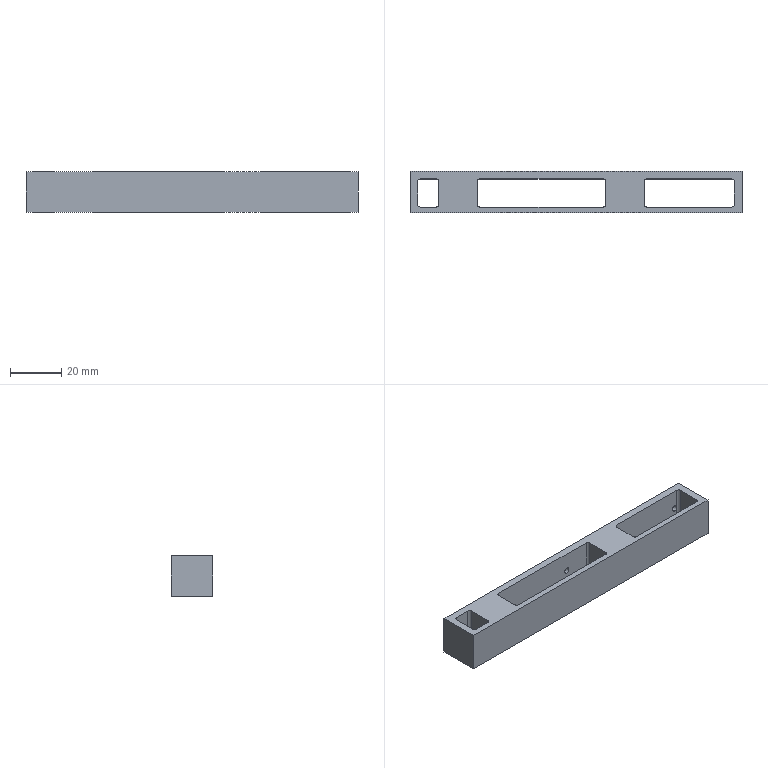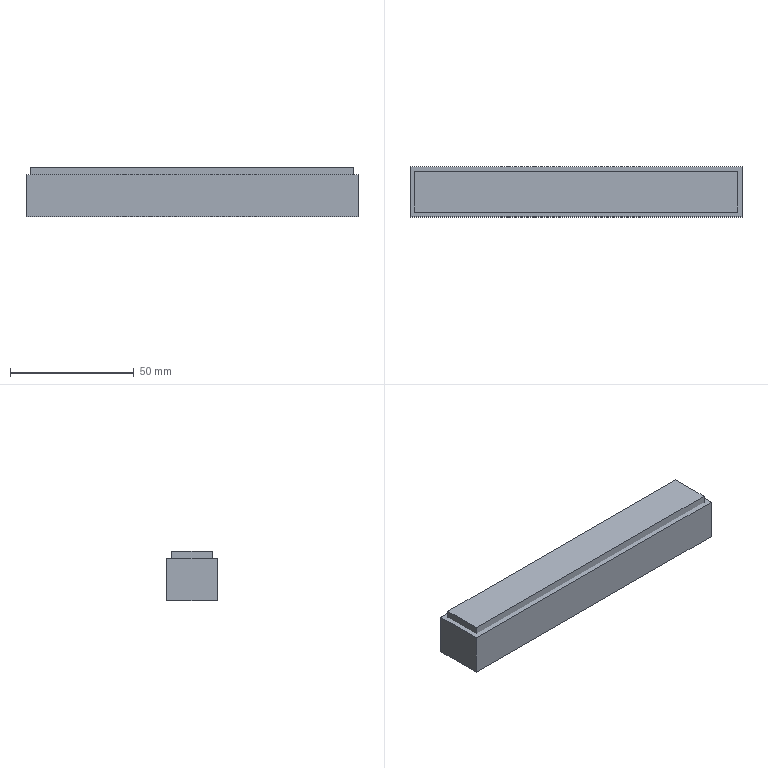CAM job | NX | 3+2 milling, drilling | part box 130 x 16.2 x 16 mm | stock box 134 x 20.2 x 20 mm
Tools:
number,name,description,diameter,corner_radius,flute_length,length,flutes
1,D63,Milling Tool-5 Parameters,63.0,0.0,50.0,75.0,2
10,D10,Milling Tool-5 Parameters,10.0,0.0,50.0,75.0,2
7,D6A45,Milling Tool-5 Parameters,6.0,0.0,50.0,75.0,2
6,D6,Milling Tool-5 Parameters,6.0,0.0,50.0,75.0,2
2,D2,Milling Tool-5 Parameters,2.0,0.0,50.0,75.0,2
12,2.6ZT,Drilling Tool,2.4,0.0,35.0,50.0,2
13,M3,Milling Tool-5 Parameters,2.4,0.0,50.0,75.0,2
Operations:
program,operation,operation_type,tool,method,geometry_group,spindle_rpm,surface_speed,feed_per_tooth,feed_cut,feed_plunge,cut_length_mm,path_length_mm,cut_time_min,machine_time_min
1,FLOOR_WALL,VolumeBased25DMillingOperation,D63,METHOD,A,6500.0,1286.0,0.0962,1250.0,100.0,209.0,263.0,0.1672,0.1726
1,ZLEVEL_PROFILE,ZLevelMilling,D10,METHOD,A,9500.0,298.0,0.1316,2500.0,1000.0,5297.797,5370.797,2.148,2.155
1,ZLEVEL_PROFILE_COPY,ZLevelMilling,D10,METHOD,A,9500.0,298.0,0.0632,1200.0,1000.0,332.154,421.154,0.2775,0.2864
1,ZLEVEL_PROFILE_COPY_1,ZLevelMilling,D6,METHOD,A,9500.0,298.0,0.1316,2500.0,1000.0,6107.215,6437.606,2.511,2.544
1,ZLEVEL_PROFILE_COPY_COPY,ZLevelMilling,D6,METHOD,A,9500.0,298.0,0.0632,1200.0,1000.0,1186.162,1578.754,1.041,1.08
1,ZLEVEL_PROFILE_COPY_1_COPY,ZLevelMilling,D2,METHOD,A,9500.0,59.0,0.1053,2000.0,1000.0,12726.374,18962.296,7.606,8.23
1,PLANAR_MILL,PlanarMilling,D6A45,METHOD,A,9500.0,179.0,0.0658,1250.0,100.0,548.921,894.082,0.4391,0.4737
2,FLOOR_WALL_COPY,VolumeBased25DMillingOperation,D63,METHOD,B,6500.0,1286.0,0.0962,1250.0,100.0,820.0,1621.001,0.656,0.7361
2,PLANAR_MILL_COPY,PlanarMilling,D6A45,METHOD,B,9500.0,179.0,0.0658,1250.0,100.0,548.921,892.823,0.4391,0.4735
3,DRILLING,Operation,D6A45,METHOD,C,5000.0,94.0,0.025,250.0,0.0,13.8,273.113,0.0552,0.0811
3,DRILLING_COPY,Operation,2.6ZT,METHOD,C,2000.0,16.0,0.03,120.0,0.0,24.663,294.839,0.2055,0.2325
3,DRILLING_COPY_COPY,Operation,M3,METHOD,C,300.0,2.0,0.0008,0.5,0.0,19.5,284.513,39.0,39.026